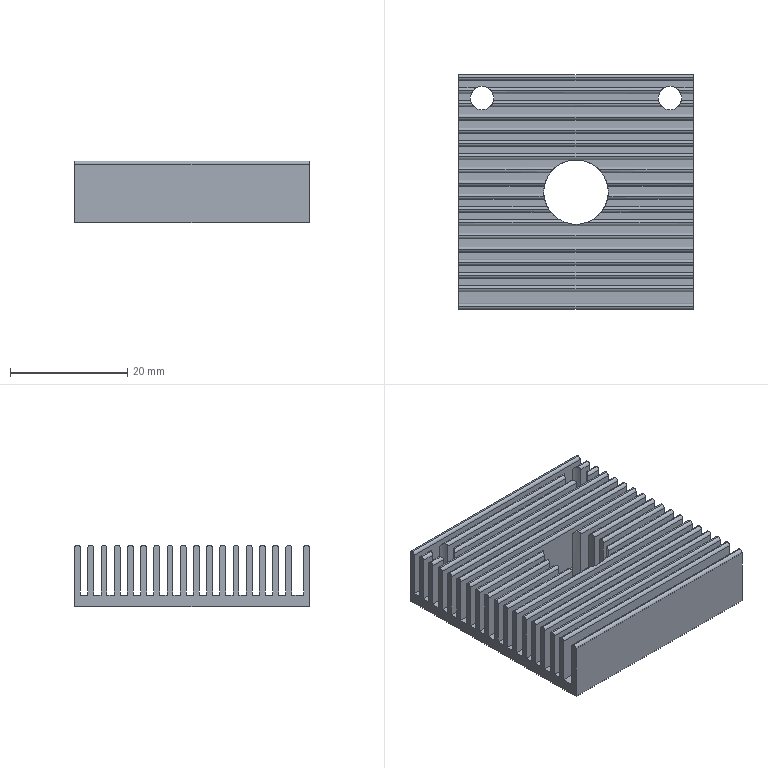Part | SolidWorks | features ICE 2, Extrusion 1, Fillet 1, LPattern 1, MirrorPattern 1 | 1 solid | 139 faces | box 40 x 40 x 10.5 mm | volume 8547 mm3 | plane 80 | cylinder 59 | commonest cylinder face diameters 1 x53 4 x4 11 x2